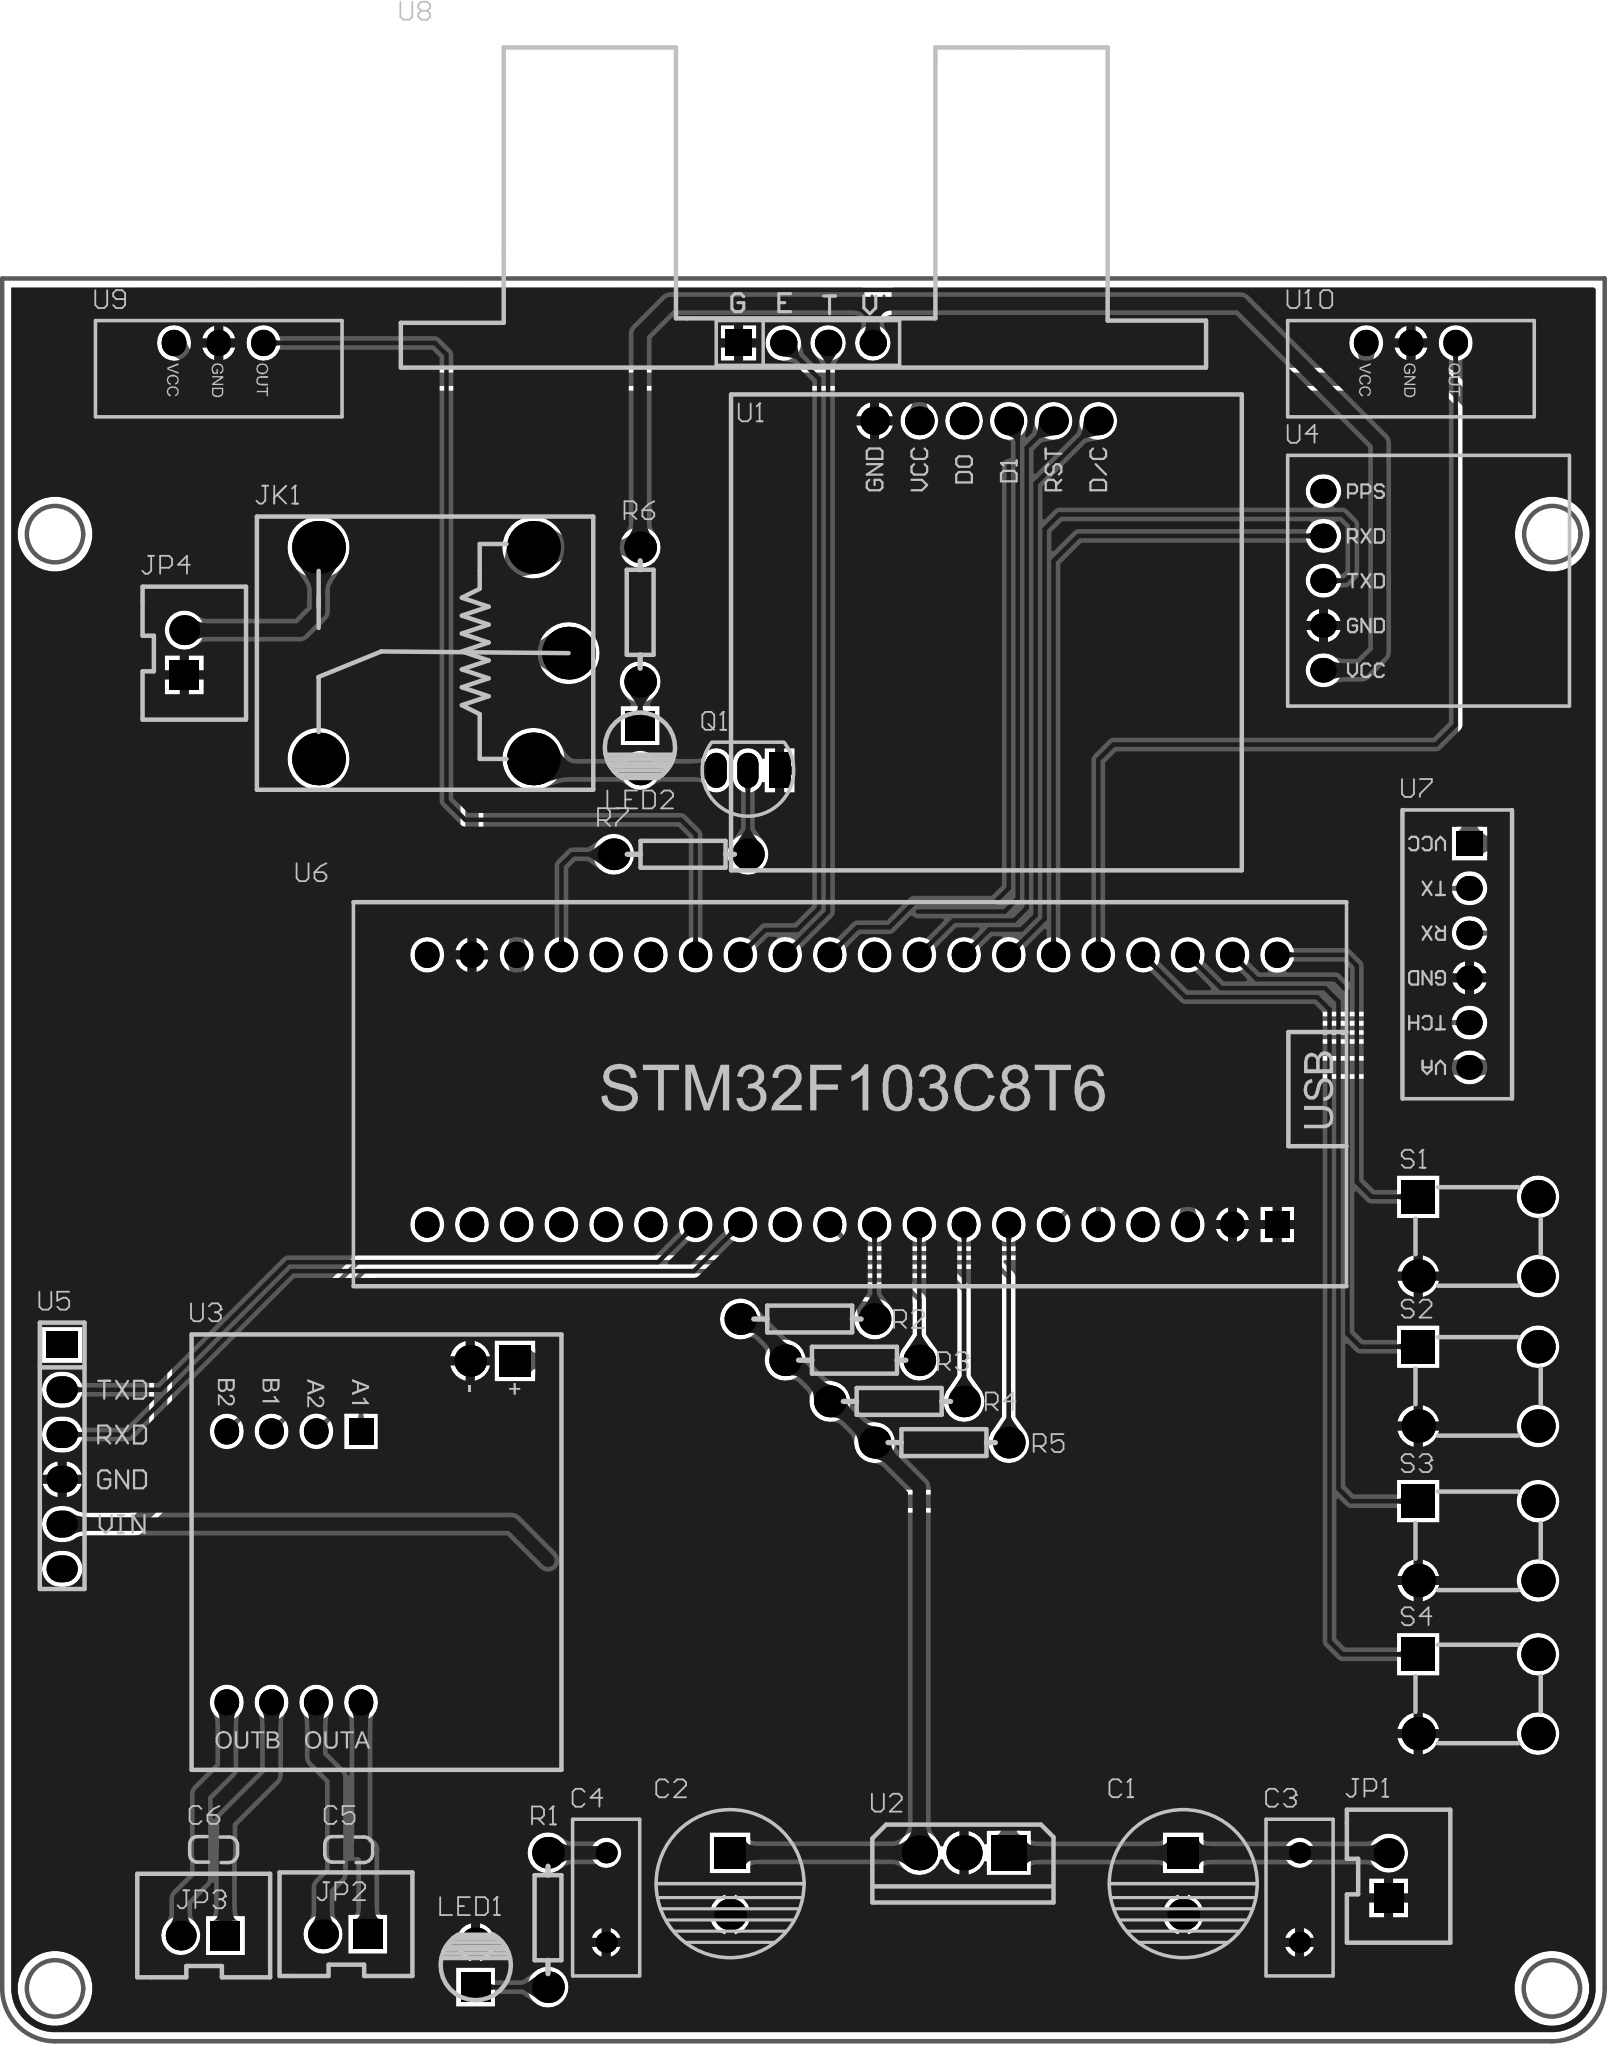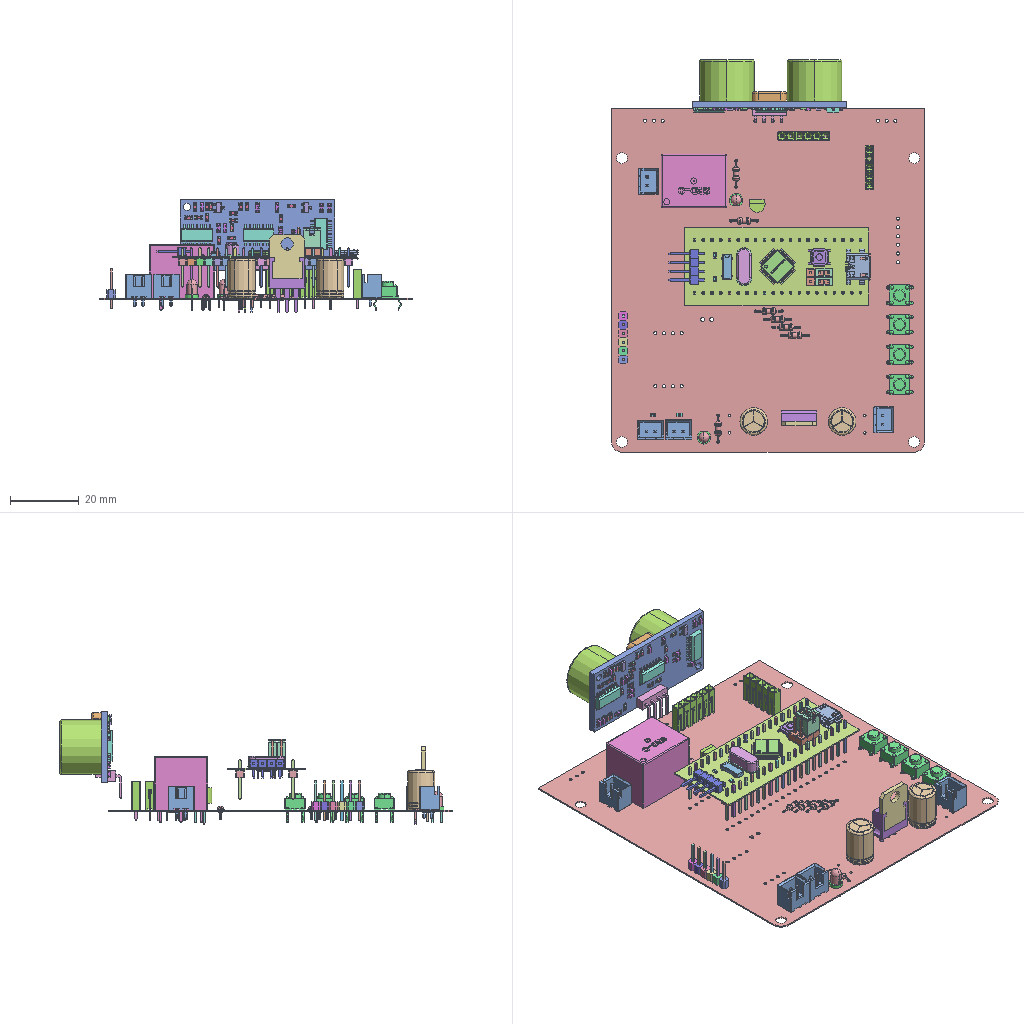Circuit board layout | Altium Designer | box 91 x 114.1 x 32.6 mm
Layer stack:
# Altium Designer layer stack of  (unit mm; dielectric type: 0 none, 1 core, 2 prepreg, 3 surface material)
index,name,kind,layer,copper_thickness_mm,dielectric_type,dielectric_thickness_mm,dielectric_material,dielectric_constant
0,Top Paste,other,,,,,,
1,Top Overlay,other,,,,,,
2,Top Solder,dielectric,,,3,0.0102,Solder Resist,3.5
3,Top Layer,copper,Top Layer,0.0356,,,,
4,Dielectric 1,dielectric,,,0,0.32,FR-4,4.8
5,Bottom Layer,copper,Bottom Layer,0.0356,,,,
6,Bottom Solder,dielectric,,,3,0.0102,Solder Resist,3.5
7,Bottom Overlay,other,,,,,,
8,Bottom Paste,other,,,,,,
# drill layer pairs: low layer,high layer
drill_pair,Top Layer,Bottom Layer
Part placement:
Designator,Comment,Layer,Footprint,Center-X(mm),Center-Y(mm),Rotation
U10,IR pair,TopLayer,火焰传感器,152.349,143.205,270
U9,IR pair,TopLayer,火焰传感器,84.658,143.205,270
U8,HC-SR04,TopLayer,超声波MODE,117.983,143.205,0
U7,AS608,TopLayer,AS608,155.677,108.458,180
U6,STM32F103,TopLayer,STM32FF103,120.625,100.843,90
U5,Header 6,TopLayer,Pin_HDR1X6/2.54mm-S,75.768,80.01,0
U4,GPS module,TopLayer,GPS,147.381,129.718,0
U3,MX1508,TopLayer,马达驱动芯片,93.295,75.771,270
U2,LM7805,TopLayer,TO220A,126.975,57.551,180
U1,OLED-SPI,TopLayer,OLED-SPI,128.245,138.786,0
S4,BUTTOM,TopLayer,DIP-6X6X5,156.163,66.563,0
S3,BUTTOM,TopLayer,DIP-6X6X5,156.163,75.25,0
S2,BUTTOM,TopLayer,DIP-6X6X5,156.163,84.013,0
S1,BUTTOM,TopLayer,DIP-6X6X5,156.163,92.517,0
R7,10K,TopLayer,AXIAL0.3,110.893,114.198,0
R6,1K,TopLayer,AXIAL0.3,108.585,127.799,90
R5,10K,TopLayer,AXIAL0.3,125.705,80.823,0
R4,10K,TopLayer,AXIAL0.3,123.165,83.16,0
R3,10K,TopLayer,AXIAL0.3,120.625,85.496,0
R2,10K,TopLayer,AXIAL0.3,118.085,87.833,0
R1,1K,TopLayer,AXIAL0.3,103.353,53.741,90
Q1,9013,TopLayer,TO-92A,114.703,118.959,180
LED2,LED,TopLayer,LED_3MM-B,108.585,120.229,270
LED1,LED,TopLayer,LED_3MM-B,99.238,51.201,90
JP4,2PIN,TopLayer,XH2.54-LI-2P,82.702,125.644,90
JP3,2PIN,TopLayer,XH2.54-LI-2P,83.769,52.857,180
JP2,2PIN,TopLayer,XH2.54-LI-2P,91.846,52.934,180
JP1,2PIN,TopLayer,XH2.54-LI-2P,151.079,56.261,90
JK1,SRD-05VDC-SL-C,TopLayer,SRD-C_B,97.422,125.609,180
C6,10uF,TopLayer,0603C,84.366,57.747,0
C5,10uF,TopLayer,0603C,92.037,57.747,0
C4,104,TopLayer,RAD-0.2,106.655,55.011,90
C3,104,TopLayer,RAD-0.2,146.025,55.011,90
C2,220uF/25V,TopLayer,DIP-EC3.5X8X11.5,113.69,55.801,270
C1,220uF/25V,TopLayer,DIP-EC3.5X8X11.5,139.421,55.801,270
Pad and via stacks:
# Altium Designer via and pad stacks of  (unit mm). Each distinct definition once, with the count of objects using it.
# via: kind,start_layer,end_layer,hole_mm,diameter_mm,mode(0 simple;1 top-mid-bottom;2 full stack),diameter_per_layer,count,example_net
# pad: kind,layer,hole_mm,hole_type(0 round;1 square;2 slot),plating,top_size,top_shape(1 round;2 rect;3 octagon;9 rounded rect),mid_size,bottom_size,mode,footprint,size_per_layer,count,example
pad,Multi-Layer,0.9,0,plated,1.7x1.7,1,1.7x1.7,1.7x1.7,0,LED 3MM-B,,2,LED2.2
pad,Multi-Layer,0.9,0,plated,1.7x1.7,2,1.7x1.7,1.7x1.7,0,LED 3MM-B,,2,LED2.1
pad,Multi-Layer,1.143,0,plated,1.626x1.626,1,1.626x1.626,1.626x1.626,0,OLED-SPI,,6,U1.6
pad,Multi-Layer,0.8,0,plated,1.8x1.8,1,1.8x1.8,1.8x1.8,0,AXIAL0.3,,14,R4.2
pad,Multi-Layer,0.9,0,plated,1.4x1.5,1,1.4x1.5,1.4x1.5,0,STM32FF103,,39,U6.20
pad,Multi-Layer,0.9,0,plated,1.4x1.5,2,1.4x1.5,1.4x1.5,0,STM32FF103,,1,U6.1
pad,Multi-Layer,0.9,0,plated,1.7x1.7,1,1.7x1.7,1.7x1.7,0,XH2.54-LI-2P,,4,JP2.2
pad,Multi-Layer,0.9,0,plated,1.7x1.7,2,1.7x1.7,1.7x1.7,0,XH2.54-LI-2P,,4,JP2.1
pad,Multi-Layer,1.1,0,plated,2x2,1,2x2,2x2,0,TO220A,,2,U2.2
pad,Multi-Layer,1.1,0,plated,2x2,2,2x2,2x2,0,TO220A,,1,U2.1
pad,Multi-Layer,0.9,0,plated,1.8x1.8,1,1.8x1.8,1.8x1.8,0,DIP-EC3.5X8X11.5,,2,C2.2
pad,Multi-Layer,0.9,0,plated,1.8x1.8,2,1.8x1.8,1.8x1.8,0,DIP-EC3.5X8X11.5,,2,C2.1
pad,Multi-Layer,0.7,0,plated,1.2x1.2,1,1.2x1.2,1.2x1.2,0,RAD-0.2,,4,C4.2
pad,Multi-Layer,1.2,0,plated,1.8x1.8,1,1.8x1.8,1.8x1.8,0,\u00C2\u00ED\u00B4\u00EF\u00C7\u00FD\u00B6\u00AF\u00D0\u00BE\u00C6\u00AC,,1,U3.10
pad,Multi-Layer,0.9,0,plated,1.4x1.5,1,1.4x1.5,1.4x1.5,0,\u00C2\u00ED\u00B4\u00EF\u00C7\u00FD\u00B6\u00AF\u00D0\u00BE\u00C6\u00AC,,7,U3.4
pad,Multi-Layer,0.9,0,plated,1.4x1.5,2,1.4x1.5,1.4x1.5,0,\u00C2\u00ED\u00B4\u00EF\u00C7\u00FD\u00B6\u00AF\u00D0\u00BE\u00C6\u00AC,,1,U3.1
pad,Multi-Layer,1.2,0,plated,1.8x1.8,2,1.8x1.8,1.8x1.8,0,\u00C2\u00ED\u00B4\u00EF\u00C7\u00FD\u00B6\u00AF\u00D0\u00BE\u00C6\u00AC,,1,U3.9
pad,Multi-Layer,0.8128,0,plated,1.524x1.778,1,1.524x1.778,1.524x1.778,0,Pin HDR1X6/2.54mm-S,,5,U5.6
pad,Multi-Layer,0.8128,0,plated,1.524x1.778,2,1.524x1.778,1.524x1.778,0,Pin HDR1X6/2.54mm-S,,1,U5.1
pad,Multi-Layer,0.9,0,plated,1.4x1.5,1,1.4x1.5,1.4x1.5,0,GPS,,5,U4.5
pad,Multi-Layer,0.9,0,plated,1.4x1.5,2,1.4x1.5,1.4x1.5,0,AS608,,1,U7.1
pad,Multi-Layer,0.9,0,plated,1.4x1.5,1,1.4x1.5,1.4x1.5,0,AS608,,5,U7.2
pad,Multi-Layer,0.85,0,plated,1.5x1.5,1,1.5x1.5,1.5x1.5,0,\u00B3\u00AC\u00C9\u00F9\u00B2\u00A8MODE,,3,U8.3
pad,Multi-Layer,0.85,0,plated,1.5x1.5,2,1.5x1.5,1.5x1.5,0,\u00B3\u00AC\u00C9\u00F9\u00B2\u00A8MODE,,1,U8.1
pad,Multi-Layer,1.6,0,plated,3x3,1,3x3,3x3,0,SRD-C_B,,5,JK1.3
pad,Multi-Layer,1,0,plated,1.9x1.9,1,1.9x1.9,1.9x1.9,0,DIP-6X6X5,,12,S1.4
pad,Multi-Layer,1,0,plated,1.9x1.9,2,1.9x1.9,1.9x1.9,0,DIP-6X6X5,,4,S1.1
pad,Multi-Layer,0.9,0,plated,1.4x1.5,1,1.4x1.5,1.4x1.5,0,\u00BB\u00F0\u00D1\u00E6\u00B4\u00AB\u00B8\u00D0\u00C6\u00F7,,6,U10.1
pad,Multi-Layer,0.8,0,plated,2x1.2,2,2x1.2,2x1.2,0,TO-92A,,1,Q1.E
pad,Multi-Layer,0.8,0,plated,2x1.2,1,2x1.2,2x1.2,0,TO-92A,,2,Q1.B
pad,Top Layer,0,0,plated,0.762x0.762,2,0.762x0.762,0.762x0.762,0,0603C,,4,C5.2
Copper pours:
name,layer,net,type(0 solid;1 hatched;2 none)
NONET_L-01_P-001,Bottom Layer,GND,0
NONET_L-01_P-001,Top Layer,GND,0
Design rules, without the lines most boards share:
# Altium Designer design rules of  (exported by Altium Designer, unit mm)
# columns: name | kind | enabled | priority | scope1 | scope2 | descriptor | typed fields (field=value)
BoardOutlineClearance | 63 | enabled | 1 | All | All | Board Clearance Constraint (Gap=0mil) (All) |
HoleToHoleClearance | 52 | enabled | 1 | All | All | Hole To Hole Clearance (Gap=10mil) (All),(All) | gap=0.254
DiffPairsRouting | 51 | enabled | 1 | All | All | Differential Pairs Uncoupled Length using the Gap Constraints (Min=10mil) (Max=10mil) (Prefered=10mil)  and Width Constraints (Min=15mil) (Max=15mil) (Prefered=15mil) (All) |
Height | 50 | enabled | 1 | All | All | Height Constraint (Min=0mil) (Max=4000mil) (Prefered=500mil) (All) | min_height=0 max_height=101.6
SolderMaskExpansion | 13 | enabled | 1 | All | All | Solder Mask Expansion (Expansion =4mil) (All) | expansion=0.1016
PasteMaskExpansion | 14 | enabled | 1 | All | All | Paste Mask Expansion (Expansion =0mil) (All) | expansion=0
RoutingVias | 11 | enabled | 1 | All | All | Routing Via (MinHoleWidth=28mil) (MaxHoleWidth=28mil) (PreferredHoleWidth=28mil) (MinWidth=50mil) (MaxWidth=50mil) (PreferedWidth=50mil) (All) | via_min_hole=0.7112 via_max_hole=0.7112 via_preferred_diameter=1.27 via_preferred_hole=0.7112
Width | 2 | enabled | 1 | All | All | Width Constraint (Min=10mil) (Max=30mil) (Preferred=10mil) (All) |
PolygonConnect | 20 | enabled | 1 | All | All | Polygon Connect Rule(Relief Connect )(Conductor Width=20mil) (Relief Angle=90 Angle) (Entries=4) (Air Gap Width=10mil) (All),(All) | connect_style(0=relief,1=direct,2=none)=0 relief_conductor_width=0.508 relief_entries=4
PlaneConnect | 6 | enabled | 1 | All | All | Power Plane Connect Rule(Relief Connect )(Expansion=20mil) (Conductor Width=10mil) (Air Gap=10mil) (Entries=4) (All) | relief_conductor_width=0.254 relief_entries=4 relief_expansion=0.508
Clearance | 0 | enabled | 1 | All | All | Clearance Constraint (Gap=10mil) (All),(All) | gap=0.254